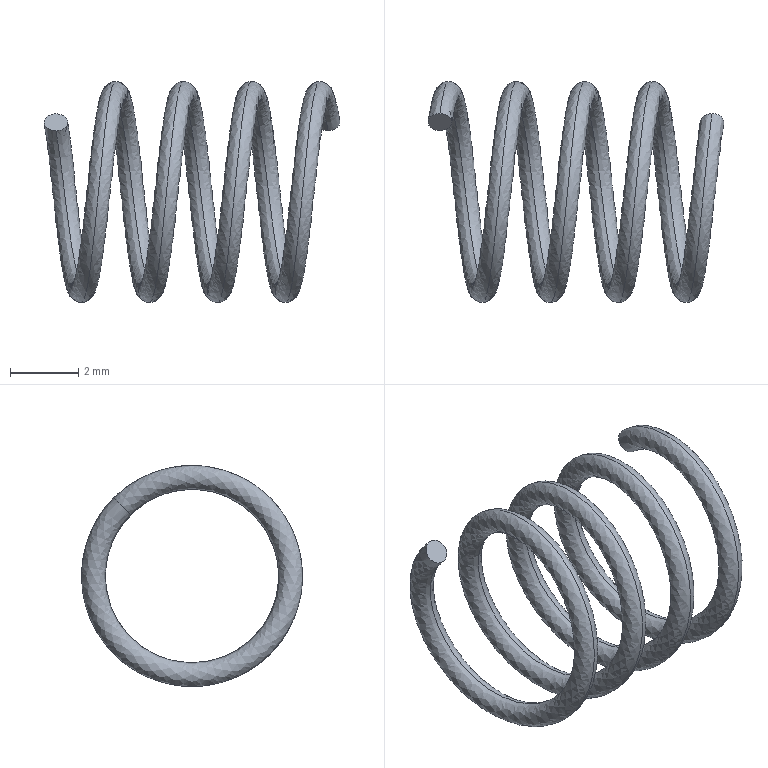Part | STEP file | High-temperature rubber spring | 1 solid | 4 faces | box 8.7 x 6.5 x 6.5 mm | volume 27.892 mm3 | spline 2 | plane 2
STEP:
#1=CARTESIAN_POINT('',(0.,0.,0.));
#2=DIRECTION('',(0.,0.,1.));
#3=DIRECTION('',(1.,0.,0.));
#4=AXIS2_PLACEMENT_3D('',#1,#2,#3);
#5=CARTESIAN_POINT('',(8.,1.803,1.803));
#6=VERTEX_POINT('',#5);
#7=CARTESIAN_POINT('',(8.,2.298,2.298));
#8=VERTEX_POINT('',#7);
#9=CARTESIAN_POINT('',(8.,1.803,1.803));
#10=CARTESIAN_POINT('',(8.7,1.803,1.803));
#11=CARTESIAN_POINT('',(8.7,2.298,2.298));
#12=CARTESIAN_POINT('',(8.,2.298,2.298));
#13=(BOUNDED_CURVE()B_SPLINE_CURVE(3,(#9,#10,#11,#12),.UNSPECIFIED.,.F.,.F.)B_SPLINE_CURVE_WITH_KNOTS((4,4),(0.,0.001094),.PIECEWISE_BEZIER_KNOTS.)CURVE()GEOMETRIC_REPRESENTATION_ITEM()RATIONAL_B_SPLINE_CURVE((1.,0.3333,0.3333,1.))REPRESENTATION_ITEM(''));
#14=CARTESIAN_POINT('',(0.,2.298,2.298));
#15=CARTESIAN_POINT('',(0.1,3.045,1.551));
#16=CARTESIAN_POINT('',(0.2,3.21,0.5084));
#17=CARTESIAN_POINT('',(0.3,3.375,-0.5346));
#18=CARTESIAN_POINT('',(0.4,2.896,-1.475));
#19=CARTESIAN_POINT('',(0.5,2.416,-2.416));
#20=CARTESIAN_POINT('',(0.6,1.475,-2.896));
#21=CARTESIAN_POINT('',(0.7,0.5346,-3.375));
#22=CARTESIAN_POINT('',(0.8,-0.5084,-3.21));
#23=CARTESIAN_POINT('',(0.9,-1.551,-3.045));
#24=CARTESIAN_POINT('',(1.,-2.298,-2.298));
#25=CARTESIAN_POINT('',(1.1,-3.045,-1.551));
#26=CARTESIAN_POINT('',(1.2,-3.21,-0.5084));
#27=CARTESIAN_POINT('',(1.3,-3.375,0.5346));
#28=CARTESIAN_POINT('',(1.4,-2.896,1.475));
#29=CARTESIAN_POINT('',(1.5,-2.416,2.416));
#30=CARTESIAN_POINT('',(1.6,-1.475,2.896));
#31=CARTESIAN_POINT('',(1.7,-0.5346,3.375));
#32=CARTESIAN_POINT('',(1.8,0.5084,3.21));
#33=CARTESIAN_POINT('',(1.9,1.551,3.045));
#34=CARTESIAN_POINT('',(2.,2.298,2.298));
#35=CARTESIAN_POINT('',(2.1,3.045,1.551));
#36=CARTESIAN_POINT('',(2.2,3.21,0.5084));
#37=CARTESIAN_POINT('',(2.3,3.375,-0.5346));
#38=CARTESIAN_POINT('',(2.4,2.896,-1.475));
#39=CARTESIAN_POINT('',(2.5,2.416,-2.416));
#40=CARTESIAN_POINT('',(2.6,1.475,-2.896));
#41=CARTESIAN_POINT('',(2.7,0.5346,-3.375));
#42=CARTESIAN_POINT('',(2.8,-0.5084,-3.21));
#43=CARTESIAN_POINT('',(2.9,-1.551,-3.045));
#44=CARTESIAN_POINT('',(3.,-2.298,-2.298));
#45=CARTESIAN_POINT('',(3.1,-3.045,-1.551));
#46=CARTESIAN_POINT('',(3.2,-3.21,-0.5084));
#47=CARTESIAN_POINT('',(3.3,-3.375,0.5346));
#48=CARTESIAN_POINT('',(3.4,-2.896,1.475));
#49=CARTESIAN_POINT('',(3.5,-2.416,2.416));
#50=CARTESIAN_POINT('',(3.6,-1.475,2.896));
#51=CARTESIAN_POINT('',(3.7,-0.5346,3.375));
#52=CARTESIAN_POINT('',(3.8,0.5084,3.21));
#53=CARTESIAN_POINT('',(3.9,1.551,3.045));
#54=CARTESIAN_POINT('',(4.,2.298,2.298));
#55=CARTESIAN_POINT('',(4.1,3.045,1.551));
#56=CARTESIAN_POINT('',(4.2,3.21,0.5084));
#57=CARTESIAN_POINT('',(4.3,3.375,-0.5346));
#58=CARTESIAN_POINT('',(4.4,2.896,-1.475));
#59=CARTESIAN_POINT('',(4.5,2.416,-2.416));
#60=CARTESIAN_POINT('',(4.6,1.475,-2.896));
#61=CARTESIAN_POINT('',(4.7,0.5346,-3.375));
#62=CARTESIAN_POINT('',(4.8,-0.5084,-3.21));
#63=CARTESIAN_POINT('',(4.9,-1.551,-3.045));
#64=CARTESIAN_POINT('',(5.,-2.298,-2.298));
#65=CARTESIAN_POINT('',(5.1,-3.045,-1.551));
#66=CARTESIAN_POINT('',(5.2,-3.21,-0.5084));
#67=CARTESIAN_POINT('',(5.3,-3.375,0.5346));
#68=CARTESIAN_POINT('',(5.4,-2.896,1.475));
#69=CARTESIAN_POINT('',(5.5,-2.416,2.416));
#70=CARTESIAN_POINT('',(5.6,-1.475,2.896));
#71=CARTESIAN_POINT('',(5.7,-0.5346,3.375));
#72=CARTESIAN_POINT('',(5.8,0.5084,3.21));
#73=CARTESIAN_POINT('',(5.9,1.551,3.045));
#74=CARTESIAN_POINT('',(6.,2.298,2.298));
#75=CARTESIAN_POINT('',(6.1,3.045,1.551));
#76=CARTESIAN_POINT('',(6.2,3.21,0.5084));
#77=CARTESIAN_POINT('',(6.3,3.375,-0.5346));
#78=CARTESIAN_POINT('',(6.4,2.896,-1.475));
#79=CARTESIAN_POINT('',(6.5,2.416,-2.416));
#80=CARTESIAN_POINT('',(6.6,1.475,-2.896));
#81=CARTESIAN_POINT('',(6.7,0.5346,-3.375));
#82=CARTESIAN_POINT('',(6.8,-0.5084,-3.21));
#83=CARTESIAN_POINT('',(6.9,-1.551,-3.045));
#84=CARTESIAN_POINT('',(7.,-2.298,-2.298));
#85=CARTESIAN_POINT('',(7.1,-3.045,-1.551));
#86=CARTESIAN_POINT('',(7.2,-3.21,-0.5084));
#87=CARTESIAN_POINT('',(7.3,-3.375,0.5346));
#88=CARTESIAN_POINT('',(7.4,-2.896,1.475));
#89=CARTESIAN_POINT('',(7.5,-2.416,2.416));
#90=CARTESIAN_POINT('',(7.6,-1.475,2.896));
#91=CARTESIAN_POINT('',(7.7,-0.5346,3.375));
#92=CARTESIAN_POINT('',(7.8,0.5084,3.21));
#93=CARTESIAN_POINT('',(7.9,1.551,3.045));
#94=CARTESIAN_POINT('',(8.,2.298,2.298));
#95=CARTESIAN_POINT('',(0.7,2.298,2.298));
#96=CARTESIAN_POINT('',(0.8,3.045,1.551));
#97=CARTESIAN_POINT('',(0.9,3.21,0.5084));
#98=CARTESIAN_POINT('',(1.,3.375,-0.5346));
#99=CARTESIAN_POINT('',(1.1,2.896,-1.475));
#100=CARTESIAN_POINT('',(1.2,2.416,-2.416));
#101=CARTESIAN_POINT('',(1.3,1.475,-2.896));
#102=CARTESIAN_POINT('',(1.4,0.5346,-3.375));
#103=CARTESIAN_POINT('',(1.5,-0.5084,-3.21));
#104=CARTESIAN_POINT('',(1.6,-1.551,-3.045));
#105=CARTESIAN_POINT('',(1.7,-2.298,-2.298));
#106=CARTESIAN_POINT('',(1.8,-3.045,-1.551));
#107=CARTESIAN_POINT('',(1.9,-3.21,-0.5084));
#108=CARTESIAN_POINT('',(2.,-3.375,0.5346));
#109=CARTESIAN_POINT('',(2.1,-2.896,1.475));
#110=CARTESIAN_POINT('',(2.2,-2.416,2.416));
#111=CARTESIAN_POINT('',(2.3,-1.475,2.896));
#112=CARTESIAN_POINT('',(2.4,-0.5346,3.375));
#113=CARTESIAN_POINT('',(2.5,0.5084,3.21));
#114=CARTESIAN_POINT('',(2.6,1.551,3.045));
#115=CARTESIAN_POINT('',(2.7,2.298,2.298));
#116=CARTESIAN_POINT('',(2.8,3.045,1.551));
#117=CARTESIAN_POINT('',(2.9,3.21,0.5084));
#118=CARTESIAN_POINT('',(3.,3.375,-0.5346));
#119=CARTESIAN_POINT('',(3.1,2.896,-1.475));
#120=CARTESIAN_POINT('',(3.2,2.416,-2.416));
#121=CARTESIAN_POINT('',(3.3,1.475,-2.896));
#122=CARTESIAN_POINT('',(3.4,0.5346,-3.375));
#123=CARTESIAN_POINT('',(3.5,-0.5084,-3.21));
#124=CARTESIAN_POINT('',(3.6,-1.551,-3.045));
#125=CARTESIAN_POINT('',(3.7,-2.298,-2.298));
#126=CARTESIAN_POINT('',(3.8,-3.045,-1.551));
#127=CARTESIAN_POINT('',(3.9,-3.21,-0.5084));
#128=CARTESIAN_POINT('',(4.,-3.375,0.5346));
#129=CARTESIAN_POINT('',(4.1,-2.896,1.475));
#130=CARTESIAN_POINT('',(4.2,-2.416,2.416));
#131=CARTESIAN_POINT('',(4.3,-1.475,2.896));
#132=CARTESIAN_POINT('',(4.4,-0.5346,3.375));
#133=CARTESIAN_POINT('',(4.5,0.5084,3.21));
#134=CARTESIAN_POINT('',(4.6,1.551,3.045));
#135=CARTESIAN_POINT('',(4.7,2.298,2.298));
#136=CARTESIAN_POINT('',(4.8,3.045,1.551));
#137=CARTESIAN_POINT('',(4.9,3.21,0.5084));
#138=CARTESIAN_POINT('',(5.,3.375,-0.5346));
#139=CARTESIAN_POINT('',(5.1,2.896,-1.475));
#140=CARTESIAN_POINT('',(5.2,2.416,-2.416));
#141=CARTESIAN_POINT('',(5.3,1.475,-2.896));
#142=CARTESIAN_POINT('',(5.4,0.5346,-3.375));
#143=CARTESIAN_POINT('',(5.5,-0.5084,-3.21));
#144=CARTESIAN_POINT('',(5.6,-1.551,-3.045));
#145=CARTESIAN_POINT('',(5.7,-2.298,-2.298));
#146=CARTESIAN_POINT('',(5.8,-3.045,-1.551));
#147=CARTESIAN_POINT('',(5.9,-3.21,-0.5084));
#148=CARTESIAN_POINT('',(6.,-3.375,0.5346));
#149=CARTESIAN_POINT('',(6.1,-2.896,1.475));
#150=CARTESIAN_POINT('',(6.2,-2.416,2.416));
#151=CARTESIAN_POINT('',(6.3,-1.475,2.896));
#152=CARTESIAN_POINT('',(6.4,-0.5346,3.375));
#153=CARTESIAN_POINT('',(6.5,0.5084,3.21));
#154=CARTESIAN_POINT('',(6.6,1.551,3.045));
#155=CARTESIAN_POINT('',(6.7,2.298,2.298));
#156=CARTESIAN_POINT('',(6.8,3.045,1.551));
#157=CARTESIAN_POINT('',(6.9,3.21,0.5084));
#158=CARTESIAN_POINT('',(7.,3.375,-0.5346));
#159=CARTESIAN_POINT('',(7.1,2.896,-1.475));
#160=CARTESIAN_POINT('',(7.2,2.416,-2.416));
#161=CARTESIAN_POINT('',(7.3,1.475,-2.896));
#162=CARTESIAN_POINT('',(7.4,0.5346,-3.375));
#163=CARTESIAN_POINT('',(7.5,-0.5084,-3.21));
#164=CARTESIAN_POINT('',(7.6,-1.551,-3.045));
#165=CARTESIAN_POINT('',(7.7,-2.298,-2.298));
#166=CARTESIAN_POINT('',(7.8,-3.045,-1.551));
#167=CARTESIAN_POINT('',(7.9,-3.21,-0.5084));
#168=CARTESIAN_POINT('',(8.,-3.375,0.5346));
#169=CARTESIAN_POINT('',(8.1,-2.896,1.475));
#170=CARTESIAN_POINT('',(8.2,-2.416,2.416));
#171=CARTESIAN_POINT('',(8.3,-1.475,2.896));
#172=CARTESIAN_POINT('',(8.4,-0.5346,3.375));
#173=CARTESIAN_POINT('',(8.5,0.5084,3.21));
#174=CARTESIAN_POINT('',(8.6,1.551,3.045));
#175=CARTESIAN_POINT('',(8.7,2.298,2.298));
#176=CARTESIAN_POINT('',(0.7,1.803,1.803));
#177=CARTESIAN_POINT('',(0.8,2.389,1.217));
#178=CARTESIAN_POINT('',(0.9,2.519,0.3989));
#179=CARTESIAN_POINT('',(1.,2.648,-0.4194));
#180=CARTESIAN_POINT('',(1.1,2.272,-1.158));
#181=CARTESIAN_POINT('',(1.2,1.896,-1.896));
#182=CARTESIAN_POINT('',(1.3,1.158,-2.272));
#183=CARTESIAN_POINT('',(1.4,0.4194,-2.648));
#184=CARTESIAN_POINT('',(1.5,-0.3989,-2.519));
#185=CARTESIAN_POINT('',(1.6,-1.217,-2.389));
#186=CARTESIAN_POINT('',(1.7,-1.803,-1.803));
#187=CARTESIAN_POINT('',(1.8,-2.389,-1.217));
#188=CARTESIAN_POINT('',(1.9,-2.519,-0.3989));
#189=CARTESIAN_POINT('',(2.,-2.648,0.4194));
#190=CARTESIAN_POINT('',(2.1,-2.272,1.158));
#191=CARTESIAN_POINT('',(2.2,-1.896,1.896));
#192=CARTESIAN_POINT('',(2.3,-1.158,2.272));
#193=CARTESIAN_POINT('',(2.4,-0.4194,2.648));
#194=CARTESIAN_POINT('',(2.5,0.3989,2.519));
#195=CARTESIAN_POINT('',(2.6,1.217,2.389));
#196=CARTESIAN_POINT('',(2.7,1.803,1.803));
#197=CARTESIAN_POINT('',(2.8,2.389,1.217));
#198=CARTESIAN_POINT('',(2.9,2.519,0.3989));
#199=CARTESIAN_POINT('',(3.,2.648,-0.4194));
#200=CARTESIAN_POINT('',(3.1,2.272,-1.158));
#201=CARTESIAN_POINT('',(3.2,1.896,-1.896));
#202=CARTESIAN_POINT('',(3.3,1.158,-2.272));
#203=CARTESIAN_POINT('',(3.4,0.4194,-2.648));
#204=CARTESIAN_POINT('',(3.5,-0.3989,-2.519));
#205=CARTESIAN_POINT('',(3.6,-1.217,-2.389));
#206=CARTESIAN_POINT('',(3.7,-1.803,-1.803));
#207=CARTESIAN_POINT('',(3.8,-2.389,-1.217));
#208=CARTESIAN_POINT('',(3.9,-2.519,-0.3989));
#209=CARTESIAN_POINT('',(4.,-2.648,0.4194));
#210=CARTESIAN_POINT('',(4.1,-2.272,1.158));
#211=CARTESIAN_POINT('',(4.2,-1.896,1.896));
#212=CARTESIAN_POINT('',(4.3,-1.158,2.272));
#213=CARTESIAN_POINT('',(4.4,-0.4194,2.648));
#214=CARTESIAN_POINT('',(4.5,0.3989,2.519));
#215=CARTESIAN_POINT('',(4.6,1.217,2.389));
#216=CARTESIAN_POINT('',(4.7,1.803,1.803));
#217=CARTESIAN_POINT('',(4.8,2.389,1.217));
#218=CARTESIAN_POINT('',(4.9,2.519,0.3989));
#219=CARTESIAN_POINT('',(5.,2.648,-0.4194));
#220=CARTESIAN_POINT('',(5.1,2.272,-1.158));
#221=CARTESIAN_POINT('',(5.2,1.896,-1.896));
#222=CARTESIAN_POINT('',(5.3,1.158,-2.272));
#223=CARTESIAN_POINT('',(5.4,0.4194,-2.648));
#224=CARTESIAN_POINT('',(5.5,-0.3989,-2.519));
#225=CARTESIAN_POINT('',(5.6,-1.217,-2.389));
#226=CARTESIAN_POINT('',(5.7,-1.803,-1.803));
#227=CARTESIAN_POINT('',(5.8,-2.389,-1.217));
#228=CARTESIAN_POINT('',(5.9,-2.519,-0.3989));
#229=CARTESIAN_POINT('',(6.,-2.648,0.4194));
#230=CARTESIAN_POINT('',(6.1,-2.272,1.158));
#231=CARTESIAN_POINT('',(6.2,-1.896,1.896));
#232=CARTESIAN_POINT('',(6.3,-1.158,2.272));
#233=CARTESIAN_POINT('',(6.4,-0.4194,2.648));
#234=CARTESIAN_POINT('',(6.5,0.3989,2.519));
#235=CARTESIAN_POINT('',(6.6,1.217,2.389));
#236=CARTESIAN_POINT('',(6.7,1.803,1.803));
#237=CARTESIAN_POINT('',(6.8,2.389,1.217));
#238=CARTESIAN_POINT('',(6.9,2.519,0.3989));
#239=CARTESIAN_POINT('',(7.,2.648,-0.4194));
#240=CARTESIAN_POINT('',(7.1,2.272,-1.158));
#241=CARTESIAN_POINT('',(7.2,1.896,-1.896));
#242=CARTESIAN_POINT('',(7.3,1.158,-2.272));
#243=CARTESIAN_POINT('',(7.4,0.4194,-2.648));
#244=CARTESIAN_POINT('',(7.5,-0.3989,-2.519));
#245=CARTESIAN_POINT('',(7.6,-1.217,-2.389));
#246=CARTESIAN_POINT('',(7.7,-1.803,-1.803));
#247=CARTESIAN_POINT('',(7.8,-2.389,-1.217));
#248=CARTESIAN_POINT('',(7.9,-2.519,-0.3989));
#249=CARTESIAN_POINT('',(8.,-2.648,0.4194));
#250=CARTESIAN_POINT('',(8.1,-2.272,1.158));
#251=CARTESIAN_POINT('',(8.2,-1.896,1.896));
#252=CARTESIAN_POINT('',(8.3,-1.158,2.272));
#253=CARTESIAN_POINT('',(8.4,-0.4194,2.648));
#254=CARTESIAN_POINT('',(8.5,0.3989,2.519));
#255=CARTESIAN_POINT('',(8.6,1.217,2.389));
#256=CARTESIAN_POINT('',(8.7,1.803,1.803));
#257=CARTESIAN_POINT('',(0.,1.803,1.803));
#258=CARTESIAN_POINT('',(0.1,2.389,1.217));
#259=CARTESIAN_POINT('',(0.2,2.519,0.3989));
#260=CARTESIAN_POINT('',(0.3,2.648,-0.4194));
#261=CARTESIAN_POINT('',(0.4,2.272,-1.158));
#262=CARTESIAN_POINT('',(0.5,1.896,-1.896));
#263=CARTESIAN_POINT('',(0.6,1.158,-2.272));
#264=CARTESIAN_POINT('',(0.7,0.4194,-2.648));
#265=CARTESIAN_POINT('',(0.8,-0.3989,-2.519));
#266=CARTESIAN_POINT('',(0.9,-1.217,-2.389));
#267=CARTESIAN_POINT('',(1.,-1.803,-1.803));
#268=CARTESIAN_POINT('',(1.1,-2.389,-1.217));
#269=CARTESIAN_POINT('',(1.2,-2.519,-0.3989));
#270=CARTESIAN_POINT('',(1.3,-2.648,0.4194));
#271=CARTESIAN_POINT('',(1.4,-2.272,1.158));
#272=CARTESIAN_POINT('',(1.5,-1.896,1.896));
#273=CARTESIAN_POINT('',(1.6,-1.158,2.272));
#274=CARTESIAN_POINT('',(1.7,-0.4194,2.648));
#275=CARTESIAN_POINT('',(1.8,0.3989,2.519));
#276=CARTESIAN_POINT('',(1.9,1.217,2.389));
#277=CARTESIAN_POINT('',(2.,1.803,1.803));
#278=CARTESIAN_POINT('',(2.1,2.389,1.217));
#279=CARTESIAN_POINT('',(2.2,2.519,0.3989));
#280=CARTESIAN_POINT('',(2.3,2.648,-0.4194));
#281=CARTESIAN_POINT('',(2.4,2.272,-1.158));
#282=CARTESIAN_POINT('',(2.5,1.896,-1.896));
#283=CARTESIAN_POINT('',(2.6,1.158,-2.272));
#284=CARTESIAN_POINT('',(2.7,0.4194,-2.648));
#285=CARTESIAN_POINT('',(2.8,-0.3989,-2.519));
#286=CARTESIAN_POINT('',(2.9,-1.217,-2.389));
#287=CARTESIAN_POINT('',(3.,-1.803,-1.803));
#288=CARTESIAN_POINT('',(3.1,-2.389,-1.217));
#289=CARTESIAN_POINT('',(3.2,-2.519,-0.3989));
#290=CARTESIAN_POINT('',(3.3,-2.648,0.4194));
#291=CARTESIAN_POINT('',(3.4,-2.272,1.158));
#292=CARTESIAN_POINT('',(3.5,-1.896,1.896));
#293=CARTESIAN_POINT('',(3.6,-1.158,2.272));
#294=CARTESIAN_POINT('',(3.7,-0.4194,2.648));
#295=CARTESIAN_POINT('',(3.8,0.3989,2.519));
#296=CARTESIAN_POINT('',(3.9,1.217,2.389));
#297=CARTESIAN_POINT('',(4.,1.803,1.803));
#298=CARTESIAN_POINT('',(4.1,2.389,1.217));
#299=CARTESIAN_POINT('',(4.2,2.519,0.3989));
#300=CARTESIAN_POINT('',(4.3,2.648,-0.4194));
#301=CARTESIAN_POINT('',(4.4,2.272,-1.158));
#302=CARTESIAN_POINT('',(4.5,1.896,-1.896));
#303=CARTESIAN_POINT('',(4.6,1.158,-2.272));
#304=CARTESIAN_POINT('',(4.7,0.4194,-2.648));
#305=CARTESIAN_POINT('',(4.8,-0.3989,-2.519));
#306=CARTESIAN_POINT('',(4.9,-1.217,-2.389));
#307=CARTESIAN_POINT('',(5.,-1.803,-1.803));
#308=CARTESIAN_POINT('',(5.1,-2.389,-1.217));
#309=CARTESIAN_POINT('',(5.2,-2.519,-0.3989));
#310=CARTESIAN_POINT('',(5.3,-2.648,0.4194));
#311=CARTESIAN_POINT('',(5.4,-2.272,1.158));
#312=CARTESIAN_POINT('',(5.5,-1.896,1.896));
#313=CARTESIAN_POINT('',(5.6,-1.158,2.272));
#314=CARTESIAN_POINT('',(5.7,-0.4194,2.648));
#315=CARTESIAN_POINT('',(5.8,0.3989,2.519));
#316=CARTESIAN_POINT('',(5.9,1.217,2.389));
#317=CARTESIAN_POINT('',(6.,1.803,1.803));
#318=CARTESIAN_POINT('',(6.1,2.389,1.217));
#319=CARTESIAN_POINT('',(6.2,2.519,0.3989));
#320=CARTESIAN_POINT('',(6.3,2.648,-0.4194));
#321=CARTESIAN_POINT('',(6.4,2.272,-1.158));
#322=CARTESIAN_POINT('',(6.5,1.896,-1.896));
#323=CARTESIAN_POINT('',(6.6,1.158,-2.272));
#324=CARTESIAN_POINT('',(6.7,0.4194,-2.648));
#325=CARTESIAN_POINT('',(6.8,-0.3989,-2.519));
#326=CARTESIAN_POINT('',(6.9,-1.217,-2.389));
#327=CARTESIAN_POINT('',(7.,-1.803,-1.803));
#328=CARTESIAN_POINT('',(7.1,-2.389,-1.217));
#329=CARTESIAN_POINT('',(7.2,-2.519,-0.3989));
#330=CARTESIAN_POINT('',(7.3,-2.648,0.4194));
#331=CARTESIAN_POINT('',(7.4,-2.272,1.158));
#332=CARTESIAN_POINT('',(7.5,-1.896,1.896));
#333=CARTESIAN_POINT('',(7.6,-1.158,2.272));
#334=CARTESIAN_POINT('',(7.7,-0.4194,2.648));
#335=CARTESIAN_POINT('',(7.8,0.3989,2.519));
#336=CARTESIAN_POINT('',(7.9,1.217,2.389));
#337=CARTESIAN_POINT('',(8.,1.803,1.803));
#338=(BOUNDED_SURFACE()B_SPLINE_SURFACE(3,2,((#14,#15,#16,#17,#18,#19,#20,#21,#22,#23,#24,#25,#26,#27,#28,#29,#30,#31,#32,#33,#34,#35,#36,#37,#38,#39,#40,#41,#42,#43,#44,#45,#46,#47,#48,#49,#50,#51,#52,#53,#54,#55,#56,#57,#58,#59,#60,#61,#62,#63,#64,#65,#66,#67,#68,#69,#70,#71,#72,#73,#74,#75,#76,#77,#78,#79,#80,#81,#82,#83,#84,#85,#86,#87,#88,#89,#90,#91,#92,#93,#94),(#95,#96,#97,#98,#99,#100,#101,#102,#103,#104,#105,#106,#107,#108,#109,#110,#111,#112,#113,#114,#115,#116,#117,#118,#119,#120,#121,#122,#123,#124,#125,#126,#127,#128,#129,#130,#131,#132,#133,#134,#135,#136,#137,#138,#139,#140,#141,#142,#143,#144,#145,#146,#147,#148,#149,#150,#151,#152,#153,#154,#155,#156,#157,#158,#159,#160,#161,#162,#163,#164,#165,#166,#167,#168,#169,#170,#171,#172,#173,#174,#175),(#176,#177,#178,#179,#180,#181,#182,#183,#184,#185,#186,#187,#188,#189,#190,#191,#192,#193,#194,#195,#196,#197,#198,#199,#200,#201,#202,#203,#204,#205,#206,#207,#208,#209,#210,#211,#212,#213,#214,#215,#216,#217,#218,#219,#220,#221,#222,#223,#224,#225,#226,#227,#228,#229,#230,#231,#232,#233,#234,#235,#236,#237,#238,#239,#240,#241,#242,#243,#244,#245,#246,#247,#248,#249,#250,#251,#252,#253,#254,#255,#256),(#257,#258,#259,#260,#261,#262,#263,#264,#265,#266,#267,#268,#269,#270,#271,#272,#273,#274,#275,#276,#277,#278,#279,#280,#281,#282,#283,#284,#285,#286,#287,#288,#289,#290,#291,#292,#293,#294,#295,#296,#297,#298,#299,#300,#301,#302,#303,#304,#305,#306,#307,#308,#309,#310,#311,#312,#313,#314,#315,#316,#317,#318,#319,#320,#321,#322,#323,#324,#325,#326,#327,#328,#329,#330,#331,#332,#333,#334,#335,#336,#337)),.UNSPECIFIED.,.F.,.F.,.F.)B_SPLINE_SURFACE_WITH_KNOTS((4,4),(3,2,2,2,2,2,2,2,2,2,2,2,2,2,2,2,2,2,2,2,2,2,2,2,2,2,2,2,2,2,2,2,2,2,2,2,2,2,2,2,3),(0.,0.5),(0.,0.025,0.05,0.075,0.1,0.125,0.15,0.175,0.2,0.225,0.25,0.275,0.3,0.325,0.35,0.375,0.4,0.425,0.45,0.475,0.5,0.525,0.55,0.575,0.6,0.625,0.65,0.675,0.7,0.725,0.75,0.775,0.8,0.825,0.85,0.875,0.9,0.925,0.95,0.975,1.),.PIECEWISE_BEZIER_KNOTS.)GEOMETRIC_REPRESENTATION_ITEM()RATIONAL_B_SPLINE_SURFACE(((1.,0.9511,1.,0.9511,1.,0.9511,1.,0.9511,1.,0.9511,1.,0.9511,1.,0.9511,1.,0.9511,1.,0.9511,1.,0.9511,1.,0.9511,1.,0.9511,1.,0.9511,1.,0.9511,1.,0.9511,1.,0.9511,1.,0.9511,1.,0.9511,1.,0.9511,1.,0.9511,1.,0.9511,1.,0.9511,1.,0.9511,1.,0.9511,1.,0.9511,1.,0.9511,1.,0.9511,1.,0.9511,1.,0.9511,1.,0.9511,1.,0.9511,1.,0.9511,1.,0.9511,1.,0.9511,1.,0.9511,1.,0.9511,1.,0.9511,1.,0.9511,1.,0.9511,1.,0.9511,1.),(0.3333,0.317,0.3333,0.317,0.3333,0.317,0.3333,0.317,0.3333,0.317,0.3333,0.317,0.3333,0.317,0.3333,0.317,0.3333,0.317,0.3333,0.317,0.3333,0.317,0.3333,0.317,0.3333,0.317,0.3333,0.317,0.3333,0.317,0.3333,0.317,0.3333,0.317,0.3333,0.317,0.3333,0.317,0.3333,0.317,0.3333,0.317,0.3333,0.317,0.3333,0.317,0.3333,0.317,0.3333,0.317,0.3333,0.317,0.3333,0.317,0.3333,0.317,0.3333,0.317,0.3333,0.317,0.3333,0.317,0.3333,0.317,0.3333,0.317,0.3333,0.317,0.3333,0.317,0.3333,0.317,0.3333,0.317,0.3333,0.317,0.3333,0.317,0.3333,0.317,0.3333),(0.3333,0.317,0.3333,0.317,0.3333,0.317,0.3333,0.317,0.3333,0.317,0.3333,0.317,0.3333,0.317,0.3333,0.317,0.3333,0.317,0.3333,0.317,0.3333,0.317,0.3333,0.317,0.3333,0.317,0.3333,0.317,0.3333,0.317,0.3333,0.317,0.3333,0.317,0.3333,0.317,0.3333,0.317,0.3333,0.317,0.3333,0.317,0.3333,0.317,0.3333,0.317,0.3333,0.317,0.3333,0.317,0.3333,0.317,0.3333,0.317,0.3333,0.317,0.3333,0.317,0.3333,0.317,0.3333,0.317,0.3333,0.317,0.3333,0.317,0.3333,0.317,0.3333,0.317,0.3333,0.317,0.3333,0.317,0.3333,0.317,0.3333,0.317,0.3333,0.317,0.3333),(1.,0.9511,1.,0.9511,1.,0.9511,1.,0.9511,1.,0.9511,1.,0.9511,1.,0.9511,1.,0.9511,1.,0.9511,1.,0.9511,1.,0.9511,1.,0.9511,1.,0.9511,1.,0.9511,1.,0.9511,1.,0.9511,1.,0.9511,1.,0.9511,1.,0.9511,1.,0.9511,1.,0.9511,1.,0.9511,1.,0.9511,1.,0.9511,1.,0.9511,1.,0.9511,1.,0.9511,1.,0.9511,1.,0.9511,1.,0.9511,1.,0.9511,1.,0.9511,1.,0.9511,1.,0.9511,1.,0.9511,1.,0.9511,1.,0.9511,1.,0.9511,1.,0.9511,1.,0.9511,1.)))REPRESENTATION_ITEM('')SURFACE());
#339=CARTESIAN_POINT('',(0.5,1.));
#340=CARTESIAN_POINT('',(0.,1.));
#341=B_SPLINE_CURVE_WITH_KNOTS('',1,(#339,#340),.UNSPECIFIED.,.F.,.F.,(2,2),(0.,0.001094),.PIECEWISE_BEZIER_KNOTS.);
#342=(GEOMETRIC_REPRESENTATION_CONTEXT(2)PARAMETRIC_REPRESENTATION_CONTEXT()REPRESENTATION_CONTEXT('',''));
#343=DEFINITIONAL_REPRESENTATION('',(#341),#342);
#344=PCURVE('',#338,#343);
#345=CARTESIAN_POINT('',(7.646,2.301,2.301));
#346=DIRECTION('',(0.,-0.7071,0.7071));
#347=DIRECTION('',(0.,-0.7071,-0.7071));
#348=AXIS2_PLACEMENT_3D('',#345,#346,#347);
#349=PLANE('',#348);
#350=CARTESIAN_POINT('',(0.7042,0.3542));
#351=CARTESIAN_POINT('',(0.7042,1.054));
#352=CARTESIAN_POINT('',(0.0042,1.054));
#353=CARTESIAN_POINT('',(0.0042,0.3542));
#354=(BOUNDED_CURVE()B_SPLINE_CURVE(3,(#350,#351,#352,#353),.UNSPECIFIED.,.F.,.F.)B_SPLINE_CURVE_WITH_KNOTS((4,4),(0.,0.001094),.PIECEWISE_BEZIER_KNOTS.)CURVE()GEOMETRIC_REPRESENTATION_ITEM()RATIONAL_B_SPLINE_CURVE((1.,0.3333,0.3333,1.))REPRESENTATION_ITEM(''));
#355=(GEOMETRIC_REPRESENTATION_CONTEXT(2)PARAMETRIC_REPRESENTATION_CONTEXT()REPRESENTATION_CONTEXT('',''));
#356=DEFINITIONAL_REPRESENTATION('',(#354),#355);
#357=PCURVE('',#349,#356);
#358=SURFACE_CURVE('',#13,(#344,#357),.PCURVE_S1.);
#359=EDGE_CURVE('',#6,#8,#358,.T.);
#360=ORIENTED_EDGE('',*,*,#359,.T.);
#361=CARTESIAN_POINT('',(0.,2.298,2.298));
#362=VERTEX_POINT('',#361);
#363=CARTESIAN_POINT('',(8.,2.298,2.298));
#364=CARTESIAN_POINT('',(7.9,1.551,3.045));
#365=CARTESIAN_POINT('',(7.8,0.5084,3.21));
#366=CARTESIAN_POINT('',(7.7,-0.5346,3.375));
#367=CARTESIAN_POINT('',(7.6,-1.475,2.896));
#368=CARTESIAN_POINT('',(7.5,-2.416,2.416));
#369=CARTESIAN_POINT('',(7.4,-2.896,1.475));
#370=CARTESIAN_POINT('',(7.3,-3.375,0.5346));
#371=CARTESIAN_POINT('',(7.2,-3.21,-0.5084));
#372=CARTESIAN_POINT('',(7.1,-3.045,-1.551));
#373=CARTESIAN_POINT('',(7.,-2.298,-2.298));
#374=CARTESIAN_POINT('',(6.9,-1.551,-3.045));
#375=CARTESIAN_POINT('',(6.8,-0.5084,-3.21));
#376=CARTESIAN_POINT('',(6.7,0.5346,-3.375));
#377=CARTESIAN_POINT('',(6.6,1.475,-2.896));
#378=CARTESIAN_POINT('',(6.5,2.416,-2.416));
#379=CARTESIAN_POINT('',(6.4,2.896,-1.475));
#380=CARTESIAN_POINT('',(6.3,3.375,-0.5346));
#381=CARTESIAN_POINT('',(6.2,3.21,0.5084));
#382=CARTESIAN_POINT('',(6.1,3.045,1.551));
#383=CARTESIAN_POINT('',(6.,2.298,2.298));
#384=CARTESIAN_POINT('',(5.9,1.551,3.045));
#385=CARTESIAN_POINT('',(5.8,0.5084,3.21));
#386=CARTESIAN_POINT('',(5.7,-0.5346,3.375));
#387=CARTESIAN_POINT('',(5.6,-1.475,2.896));
#388=CARTESIAN_POINT('',(5.5,-2.416,2.416));
#389=CARTESIAN_POINT('',(5.4,-2.896,1.475));
#390=CARTESIAN_POINT('',(5.3,-3.375,0.5346));
#391=CARTESIAN_POINT('',(5.2,-3.21,-0.5084));
#392=CARTESIAN_POINT('',(5.1,-3.045,-1.551));
#393=CARTESIAN_POINT('',(5.,-2.298,-2.298));
#394=CARTESIAN_POINT('',(4.9,-1.551,-3.045));
#395=CARTESIAN_POINT('',(4.8,-0.5084,-3.21));
#396=CARTESIAN_POINT('',(4.7,0.5346,-3.375));
#397=CARTESIAN_POINT('',(4.6,1.475,-2.896));
#398=CARTESIAN_POINT('',(4.5,2.416,-2.416));
#399=CARTESIAN_POINT('',(4.4,2.896,-1.475));
#400=CARTESIAN_POINT('',(4.3,3.375,-0.5346));
#401=CARTESIAN_POINT('',(4.2,3.21,0.5084));
#402=CARTESIAN_POINT('',(4.1,3.045,1.551));
#403=CARTESIAN_POINT('',(4.,2.298,2.298));
#404=CARTESIAN_POINT('',(3.9,1.551,3.045));
#405=CARTESIAN_POINT('',(3.8,0.5084,3.21));
#406=CARTESIAN_POINT('',(3.7,-0.5346,3.375));
#407=CARTESIAN_POINT('',(3.6,-1.475,2.896));
#408=CARTESIAN_POINT('',(3.5,-2.416,2.416));
#409=CARTESIAN_POINT('',(3.4,-2.896,1.475));
#410=CARTESIAN_POINT('',(3.3,-3.375,0.5346));
#411=CARTESIAN_POINT('',(3.2,-3.21,-0.5084));
#412=CARTESIAN_POINT('',(3.1,-3.045,-1.551));
#413=CARTESIAN_POINT('',(3.,-2.298,-2.298));
#414=CARTESIAN_POINT('',(2.9,-1.551,-3.045));
#415=CARTESIAN_POINT('',(2.8,-0.5084,-3.21));
#416=CARTESIAN_POINT('',(2.7,0.5346,-3.375));
#417=CARTESIAN_POINT('',(2.6,1.475,-2.896));
#418=CARTESIAN_POINT('',(2.5,2.416,-2.416));
#419=CARTESIAN_POINT('',(2.4,2.896,-1.475));
#420=CARTESIAN_POINT('',(2.3,3.375,-0.5346));
#421=CARTESIAN_POINT('',(2.2,3.21,0.5084));
#422=CARTESIAN_POINT('',(2.1,3.045,1.551));
#423=CARTESIAN_POINT('',(2.,2.298,2.298));
#424=CARTESIAN_POINT('',(1.9,1.551,3.045));
#425=CARTESIAN_POINT('',(1.8,0.5084,3.21));
#426=CARTESIAN_POINT('',(1.7,-0.5346,3.375));
#427=CARTESIAN_POINT('',(1.6,-1.475,2.896));
#428=CARTESIAN_POINT('',(1.5,-2.416,2.416));
#429=CARTESIAN_POINT('',(1.4,-2.896,1.475));
#430=CARTESIAN_POINT('',(1.3,-3.375,0.5346));
#431=CARTESIAN_POINT('',(1.2,-3.21,-0.5084));
#432=CARTESIAN_POINT('',(1.1,-3.045,-1.551));
#433=CARTESIAN_POINT('',(1.,-2.298,-2.298));
#434=CARTESIAN_POINT('',(0.9,-1.551,-3.045));
#435=CARTESIAN_POINT('',(0.8,-0.5084,-3.21));
#436=CARTESIAN_POINT('',(0.7,0.5346,-3.375));
#437=CARTESIAN_POINT('',(0.6,1.475,-2.896));
#438=CARTESIAN_POINT('',(0.5,2.416,-2.416));
#439=CARTESIAN_POINT('',(0.4,2.896,-1.475));
#440=CARTESIAN_POINT('',(0.3,3.375,-0.5346));
#441=CARTESIAN_POINT('',(0.2,3.21,0.5084));
#442=CARTESIAN_POINT('',(0.1,3.045,1.551));
#443=CARTESIAN_POINT('',(0.,2.298,2.298));
#444=(BOUNDED_CURVE()B_SPLINE_CURVE(2,(#363,#364,#365,#366,#367,#368,#369,#370,#371,#372,#373,#374,#375,#376,#377,#378,#379,#380,#381,#382,#383,#384,#385,#386,#387,#388,#389,#390,#391,#392,#393,#394,#395,#396,#397,#398,#399,#400,#401,#402,#403,#404,#405,#406,#407,#408,#409,#410,#411,#412,#413,#414,#415,#416,#417,#418,#419,#420,#421,#422,#423,#424,#425,#426,#427,#428,#429,#430,#431,#432,#433,#434,#435,#436,#437,#438,#439,#440,#441,#442,#443),.UNSPECIFIED.,.F.,.F.)B_SPLINE_CURVE_WITH_KNOTS((3,2,2,2,2,2,2,2,2,2,2,2,2,2,2,2,2,2,2,2,2,2,2,2,2,2,2,2,2,2,2,2,2,2,2,2,2,2,2,2,3),(0.,0.025,0.05,0.075,0.1,0.125,0.15,0.175,0.2,0.225,0.25,0.275,0.3,0.325,0.35,0.375,0.4,0.425,0.45,0.475,0.5,0.525,0.55,0.575,0.6,0.625,0.65,0.675,0.7,0.725,0.75,0.775,0.8,0.825,0.85,0.875,0.9,0.925,0.95,0.975,1.),.UNSPECIFIED.)CURVE()GEOMETRIC_REPRESENTATION_ITEM()RATIONAL_B_SPLINE_CURVE((1.,0.9511,1.,0.9511,1.,0.9511,1.,0.9511,1.,0.9511,1.,0.9511,1.,0.9511,1.,0.9511,1.,0.9511,1.,0.9511,1.,0.9511,1.,0.9511,1.,0.9511,1.,0.9511,1.,0.9511,1.,0.9511,1.,0.9511,1.,0.9511,1.,0.9511,1.,0.9511,1.,0.9511,1.,0.9511,1.,0.9511,1.,0.9511,1.,0.9511,1.,0.9511,1.,0.9511,1.,0.9511,1.,0.9511,1.,0.9511,1.,0.9511,1.,0.9511,1.,0.9511,1.,0.9511,1.,0.9511,1.,0.9511,1.,0.9511,1.,0.9511,1.,0.9511,1.,0.9511,1.))REPRESENTATION_ITEM(''));
#445=CARTESIAN_POINT('',(0.,1.));
#446=DIRECTION('',(0.,-1.));
#447=VECTOR('',#446,1.);
#448=LINE('',#445,#447);
#449=(GEOMETRIC_REPRESENTATION_CONTEXT(2)PARAMETRIC_REPRESENTATION_CONTEXT()REPRESENTATION_CONTEXT('',''));
#450=DEFINITIONAL_REPRESENTATION('',(#448),#449);
#451=PCURVE('',#338,#450);
#452=CARTESIAN_POINT('',(0.,1.803,1.803));
#453=CARTESIAN_POINT('',(0.1,2.389,1.217));
#454=CARTESIAN_POINT('',(0.2,2.519,0.3989));
#455=CARTESIAN_POINT('',(0.3,2.648,-0.4194));
#456=CARTESIAN_POINT('',(0.4,2.272,-1.158));
#457=CARTESIAN_POINT('',(0.5,1.896,-1.896));
#458=CARTESIAN_POINT('',(0.6,1.158,-2.272));
#459=CARTESIAN_POINT('',(0.7,0.4194,-2.648));
#460=CARTESIAN_POINT('',(0.8,-0.3989,-2.519));
#461=CARTESIAN_POINT('',(0.9,-1.217,-2.389));
#462=CARTESIAN_POINT('',(1.,-1.803,-1.803));
#463=CARTESIAN_POINT('',(1.1,-2.389,-1.217));
#464=CARTESIAN_POINT('',(1.2,-2.519,-0.3989));
#465=CARTESIAN_POINT('',(1.3,-2.648,0.4194));
#466=CARTESIAN_POINT('',(1.4,-2.272,1.158));
#467=CARTESIAN_POINT('',(1.5,-1.896,1.896));
#468=CARTESIAN_POINT('',(1.6,-1.158,2.272));
#469=CARTESIAN_POINT('',(1.7,-0.4194,2.648));
#470=CARTESIAN_POINT('',(1.8,0.3989,2.519));
#471=CARTESIAN_POINT('',(1.9,1.217,2.389));
#472=CARTESIAN_POINT('',(2.,1.803,1.803));
#473=CARTESIAN_POINT('',(2.1,2.389,1.217));
#474=CARTESIAN_POINT('',(2.2,2.519,0.3989));
#475=CARTESIAN_POINT('',(2.3,2.648,-0.4194));
#476=CARTESIAN_POINT('',(2.4,2.272,-1.158));
#477=CARTESIAN_POINT('',(2.5,1.896,-1.896));
#478=CARTESIAN_POINT('',(2.6,1.158,-2.272));
#479=CARTESIAN_POINT('',(2.7,0.4194,-2.648));
#480=CARTESIAN_POINT('',(2.8,-0.3989,-2.519));
#481=CARTESIAN_POINT('',(2.9,-1.217,-2.389));
#482=CARTESIAN_POINT('',(3.,-1.803,-1.803));
#483=CARTESIAN_POINT('',(3.1,-2.389,-1.217));
#484=CARTESIAN_POINT('',(3.2,-2.519,-0.3989));
#485=CARTESIAN_POINT('',(3.3,-2.648,0.4194));
#486=CARTESIAN_POINT('',(3.4,-2.272,1.158));
#487=CARTESIAN_POINT('',(3.5,-1.896,1.896));
#488=CARTESIAN_POINT('',(3.6,-1.158,2.272));
#489=CARTESIAN_POINT('',(3.7,-0.4194,2.648));
#490=CARTESIAN_POINT('',(3.8,0.3989,2.519));
#491=CARTESIAN_POINT('',(3.9,1.217,2.389));
#492=CARTESIAN_POINT('',(4.,1.803,1.803));
#493=CARTESIAN_POINT('',(4.1,2.389,1.217));
#494=CARTESIAN_POINT('',(4.2,2.519,0.3989));
#495=CARTESIAN_POINT('',(4.3,2.648,-0.4194));
#496=CARTESIAN_POINT('',(4.4,2.272,-1.158));
#497=CARTESIAN_POINT('',(4.5,1.896,-1.896));
#498=CARTESIAN_POINT('',(4.6,1.158,-2.272));
#499=CARTESIAN_POINT('',(4.7,0.4194,-2.648));
#500=CARTESIAN_POINT('',(4.8,-0.3989,-2.519));
#501=CARTESIAN_POINT('',(4.9,-1.217,-2.389));
#502=CARTESIAN_POINT('',(5.,-1.803,-1.803));
#503=CARTESIAN_POINT('',(5.1,-2.389,-1.217));
#504=CARTESIAN_POINT('',(5.2,-2.519,-0.3989));
#505=CARTESIAN_POINT('',(5.3,-2.648,0.4194));
#506=CARTESIAN_POINT('',(5.4,-2.272,1.158));
#507=CARTESIAN_POINT('',(5.5,-1.896,1.896));
#508=CARTESIAN_POINT('',(5.6,-1.158,2.272));
#509=CARTESIAN_POINT('',(5.7,-0.4194,2.648));
#510=CARTESIAN_POINT('',(5.8,0.3989,2.519));
#511=CARTESIAN_POINT('',(5.9,1.217,2.389));
#512=CARTESIAN_POINT('',(6.,1.803,1.803));
#513=CARTESIAN_POINT('',(6.1,2.389,1.217));
#514=CARTESIAN_POINT('',(6.2,2.519,0.3989));
#515=CARTESIAN_POINT('',(6.3,2.648,-0.4194));
#516=CARTESIAN_POINT('',(6.4,2.272,-1.158));
#517=CARTESIAN_POINT('',(6.5,1.896,-1.896));
#518=CARTESIAN_POINT('',(6.6,1.158,-2.272));
#519=CARTESIAN_POINT('',(6.7,0.4194,-2.648));
#520=CARTESIAN_POINT('',(6.8,-0.3989,-2.519));
#521=CARTESIAN_POINT('',(6.9,-1.217,-2.389));
#522=CARTESIAN_POINT('',(7.,-1.803,-1.803));
#523=CARTESIAN_POINT('',(7.1,-2.389,-1.217));
#524=CARTESIAN_POINT('',(7.2,-2.519,-0.3989));
#525=CARTESIAN_POINT('',(7.3,-2.648,0.4194));
#526=CARTESIAN_POINT('',(7.4,-2.272,1.158));
#527=CARTESIAN_POINT('',(7.5,-1.896,1.896));
#528=CARTESIAN_POINT('',(7.6,-1.158,2.272));
#529=CARTESIAN_POINT('',(7.7,-0.4194,2.648));
#530=CARTESIAN_POINT('',(7.8,0.3989,2.519));
#531=CARTESIAN_POINT('',(7.9,1.217,2.389));
#532=CARTESIAN_POINT('',(8.,1.803,1.803));
#533=CARTESIAN_POINT('',(-0.7,1.803,1.803));
#534=CARTESIAN_POINT('',(-0.6,2.389,1.217));
#535=CARTESIAN_POINT('',(-0.5,2.519,0.3989));
#536=CARTESIAN_POINT('',(-0.4,2.648,-0.4194));
#537=CARTESIAN_POINT('',(-0.3,2.272,-1.158));
#538=CARTESIAN_POINT('',(-0.2,1.896,-1.896));
#539=CARTESIAN_POINT('',(-0.1,1.158,-2.272));
#540=CARTESIAN_POINT('',(0.,0.4194,-2.648));
#541=CARTESIAN_POINT('',(0.1,-0.3989,-2.519));
#542=CARTESIAN_POINT('',(0.2,-1.217,-2.389));
#543=CARTESIAN_POINT('',(0.3,-1.803,-1.803));
#544=CARTESIAN_POINT('',(0.4,-2.389,-1.217));
#545=CARTESIAN_POINT('',(0.5,-2.519,-0.3989));
#546=CARTESIAN_POINT('',(0.6,-2.648,0.4194));
#547=CARTESIAN_POINT('',(0.7,-2.272,1.158));
#548=CARTESIAN_POINT('',(0.8,-1.896,1.896));
#549=CARTESIAN_POINT('',(0.9,-1.158,2.272));
#550=CARTESIAN_POINT('',(1.,-0.4194,2.648));
#551=CARTESIAN_POINT('',(1.1,0.3989,2.519));
#552=CARTESIAN_POINT('',(1.2,1.217,2.389));
#553=CARTESIAN_POINT('',(1.3,1.803,1.803));
#554=CARTESIAN_POINT('',(1.4,2.389,1.217));
#555=CARTESIAN_POINT('',(1.5,2.519,0.3989));
#556=CARTESIAN_POINT('',(1.6,2.648,-0.4194));
#557=CARTESIAN_POINT('',(1.7,2.272,-1.158));
#558=CARTESIAN_POINT('',(1.8,1.896,-1.896));
#559=CARTESIAN_POINT('',(1.9,1.158,-2.272));
#560=CARTESIAN_POINT('',(2.,0.4194,-2.648));
#561=CARTESIAN_POINT('',(2.1,-0.3989,-2.519));
#562=CARTESIAN_POINT('',(2.2,-1.217,-2.389));
#563=CARTESIAN_POINT('',(2.3,-1.803,-1.803));
#564=CARTESIAN_POINT('',(2.4,-2.389,-1.217));
#565=CARTESIAN_POINT('',(2.5,-2.519,-0.3989));
#566=CARTESIAN_POINT('',(2.6,-2.648,0.4194));
#567=CARTESIAN_POINT('',(2.7,-2.272,1.158));
#568=CARTESIAN_POINT('',(2.8,-1.896,1.896));
#569=CARTESIAN_POINT('',(2.9,-1.158,2.272));
#570=CARTESIAN_POINT('',(3.,-0.4194,2.648));
#571=CARTESIAN_POINT('',(3.1,0.3989,2.519));
#572=CARTESIAN_POINT('',(3.2,1.217,2.389));
#573=CARTESIAN_POINT('',(3.3,1.803,1.803));
#574=CARTESIAN_POINT('',(3.4,2.389,1.217));
#575=CARTESIAN_POINT('',(3.5,2.519,0.3989));
#576=CARTESIAN_POINT('',(3.6,2.648,-0.4194));
#577=CARTESIAN_POINT('',(3.7,2.272,-1.158));
#578=CARTESIAN_POINT('',(3.8,1.896,-1.896));
#579=CARTESIAN_POINT('',(3.9,1.158,-2.272));
#580=CARTESIAN_POINT('',(4.,0.4194,-2.648));
#581=CARTESIAN_POINT('',(4.1,-0.3989,-2.519));
#582=CARTESIAN_POINT('',(4.2,-1.217,-2.389));
#583=CARTESIAN_POINT('',(4.3,-1.803,-1.803));
#584=CARTESIAN_POINT('',(4.4,-2.389,-1.217));
#585=CARTESIAN_POINT('',(4.5,-2.519,-0.3989));
#586=CARTESIAN_POINT('',(4.6,-2.648,0.4194));
#587=CARTESIAN_POINT('',(4.7,-2.272,1.158));
#588=CARTESIAN_POINT('',(4.8,-1.896,1.896));
#589=CARTESIAN_POINT('',(4.9,-1.158,2.272));
#590=CARTESIAN_POINT('',(5.,-0.4194,2.648));
#591=CARTESIAN_POINT('',(5.1,0.3989,2.519));
#592=CARTESIAN_POINT('',(5.2,1.217,2.389));
#593=CARTESIAN_POINT('',(5.3,1.803,1.803));
#594=CARTESIAN_POINT('',(5.4,2.389,1.217));
#595=CARTESIAN_POINT('',(5.5,2.519,0.3989));
#596=CARTESIAN_POINT('',(5.6,2.648,-0.4194));
#597=CARTESIAN_POINT('',(5.7,2.272,-1.158));
#598=CARTESIAN_POINT('',(5.8,1.896,-1.896));
#599=CARTESIAN_POINT('',(5.9,1.158,-2.272));
#600=CARTESIAN_POINT('',(6.,0.4194,-2.648));
#601=CARTESIAN_POINT('',(6.1,-0.3989,-2.519));
#602=CARTESIAN_POINT('',(6.2,-1.217,-2.389));
#603=CARTESIAN_POINT('',(6.3,-1.803,-1.803));
#604=CARTESIAN_POINT('',(6.4,-2.389,-1.217));
#605=CARTESIAN_POINT('',(6.5,-2.519,-0.3989));
#606=CARTESIAN_POINT('',(6.6,-2.648,0.4194));
#607=CARTESIAN_POINT('',(6.7,-2.272,1.158));
#608=CARTESIAN_POINT('',(6.8,-1.896,1.896));
#609=CARTESIAN_POINT('',(6.9,-1.158,2.272));
#610=CARTESIAN_POINT('',(7.,-0.4194,2.648));
#611=CARTESIAN_POINT('',(7.1,0.3989,2.519));
#612=CARTESIAN_POINT('',(7.2,1.217,2.389));
#613=CARTESIAN_POINT('',(7.3,1.803,1.803));
#614=CARTESIAN_POINT('',(-0.7,2.298,2.298));
#615=CARTESIAN_POINT('',(-0.6,3.045,1.551));
#616=CARTESIAN_POINT('',(-0.5,3.21,0.5084));
#617=CARTESIAN_POINT('',(-0.4,3.375,-0.5346));
#618=CARTESIAN_POINT('',(-0.3,2.896,-1.475));
#619=CARTESIAN_POINT('',(-0.2,2.416,-2.416));
#620=CARTESIAN_POINT('',(-0.1,1.475,-2.896));
#621=CARTESIAN_POINT('',(0.,0.5346,-3.375));
#622=CARTESIAN_POINT('',(0.1,-0.5084,-3.21));
#623=CARTESIAN_POINT('',(0.2,-1.551,-3.045));
#624=CARTESIAN_POINT('',(0.3,-2.298,-2.298));
#625=CARTESIAN_POINT('',(0.4,-3.045,-1.551));
#626=CARTESIAN_POINT('',(0.5,-3.21,-0.5084));
#627=CARTESIAN_POINT('',(0.6,-3.375,0.5346));
#628=CARTESIAN_POINT('',(0.7,-2.896,1.475));
#629=CARTESIAN_POINT('',(0.8,-2.416,2.416));
#630=CARTESIAN_POINT('',(0.9,-1.475,2.896));
#631=CARTESIAN_POINT('',(1.,-0.5346,3.375));
#632=CARTESIAN_POINT('',(1.1,0.5084,3.21));
#633=CARTESIAN_POINT('',(1.2,1.551,3.045));
#634=CARTESIAN_POINT('',(1.3,2.298,2.298));
#635=CARTESIAN_POINT('',(1.4,3.045,1.551));
#636=CARTESIAN_POINT('',(1.5,3.21,0.5084));
#637=CARTESIAN_POINT('',(1.6,3.375,-0.5346));
#638=CARTESIAN_POINT('',(1.7,2.896,-1.475));
#639=CARTESIAN_POINT('',(1.8,2.416,-2.416));
#640=CARTESIAN_POINT('',(1.9,1.475,-2.896));
#641=CARTESIAN_POINT('',(2.,0.5346,-3.375));
#642=CARTESIAN_POINT('',(2.1,-0.5084,-3.21));
#643=CARTESIAN_POINT('',(2.2,-1.551,-3.045));
#644=CARTESIAN_POINT('',(2.3,-2.298,-2.298));
#645=CARTESIAN_POINT('',(2.4,-3.045,-1.551));
#646=CARTESIAN_POINT('',(2.5,-3.21,-0.5084));
#647=CARTESIAN_POINT('',(2.6,-3.375,0.5346));
#648=CARTESIAN_POINT('',(2.7,-2.896,1.475));
#649=CARTESIAN_POINT('',(2.8,-2.416,2.416));
#650=CARTESIAN_POINT('',(2.9,-1.475,2.896));
#651=CARTESIAN_POINT('',(3.,-0.5346,3.375));
#652=CARTESIAN_POINT('',(3.1,0.5084,3.21));
#653=CARTESIAN_POINT('',(3.2,1.551,3.045));
#654=CARTESIAN_POINT('',(3.3,2.298,2.298));
#655=CARTESIAN_POINT('',(3.4,3.045,1.551));
#656=CARTESIAN_POINT('',(3.5,3.21,0.5084));
#657=CARTESIAN_POINT('',(3.6,3.375,-0.5346));
#658=CARTESIAN_POINT('',(3.7,2.896,-1.475));
#659=CARTESIAN_POINT('',(3.8,2.416,-2.416));
#660=CARTESIAN_POINT('',(3.9,1.475,-2.896));
#661=CARTESIAN_POINT('',(4.,0.5346,-3.375));
#662=CARTESIAN_POINT('',(4.1,-0.5084,-3.21));
#663=CARTESIAN_POINT('',(4.2,-1.551,-3.045));
#664=CARTESIAN_POINT('',(4.3,-2.298,-2.298));
#665=CARTESIAN_POINT('',(4.4,-3.045,-1.551));
#666=CARTESIAN_POINT('',(4.5,-3.21,-0.5084));
#667=CARTESIAN_POINT('',(4.6,-3.375,0.5346));
#668=CARTESIAN_POINT('',(4.7,-2.896,1.475));
#669=CARTESIAN_POINT('',(4.8,-2.416,2.416));
#670=CARTESIAN_POINT('',(4.9,-1.475,2.896));
#671=CARTESIAN_POINT('',(5.,-0.5346,3.375));
#672=CARTESIAN_POINT('',(5.1,0.5084,3.21));
#673=CARTESIAN_POINT('',(5.2,1.551,3.045));
#674=CARTESIAN_POINT('',(5.3,2.298,2.298));
#675=CARTESIAN_POINT('',(5.4,3.045,1.551));
#676=CARTESIAN_POINT('',(5.5,3.21,0.5084));
#677=CARTESIAN_POINT('',(5.6,3.375,-0.5346));
#678=CARTESIAN_POINT('',(5.7,2.896,-1.475));
#679=CARTESIAN_POINT('',(5.8,2.416,-2.416));
#680=CARTESIAN_POINT('',(5.9,1.475,-2.896));
#681=CARTESIAN_POINT('',(6.,0.5346,-3.375));
#682=CARTESIAN_POINT('',(6.1,-0.5084,-3.21));
#683=CARTESIAN_POINT('',(6.2,-1.551,-3.045));
#684=CARTESIAN_POINT('',(6.3,-2.298,-2.298));
#685=CARTESIAN_POINT('',(6.4,-3.045,-1.551));
#686=CARTESIAN_POINT('',(6.5,-3.21,-0.5084));
#687=CARTESIAN_POINT('',(6.6,-3.375,0.5346));
#688=CARTESIAN_POINT('',(6.7,-2.896,1.475));
#689=CARTESIAN_POINT('',(6.8,-2.416,2.416));
#690=CARTESIAN_POINT('',(6.9,-1.475,2.896));
#691=CARTESIAN_POINT('',(7.,-0.5346,3.375));
#692=CARTESIAN_POINT('',(7.1,0.5084,3.21));
#693=CARTESIAN_POINT('',(7.2,1.551,3.045));
#694=CARTESIAN_POINT('',(7.3,2.298,2.298));
#695=CARTESIAN_POINT('',(0.,2.298,2.298));
#696=CARTESIAN_POINT('',(0.1,3.045,1.551));
#697=CARTESIAN_POINT('',(0.2,3.21,0.5084));
#698=CARTESIAN_POINT('',(0.3,3.375,-0.5346));
#699=CARTESIAN_POINT('',(0.4,2.896,-1.475));
#700=CARTESIAN_POINT('',(0.5,2.416,-2.416));
#701=CARTESIAN_POINT('',(0.6,1.475,-2.896));
#702=CARTESIAN_POINT('',(0.7,0.5346,-3.375));
#703=CARTESIAN_POINT('',(0.8,-0.5084,-3.21));
#704=CARTESIAN_POINT('',(0.9,-1.551,-3.045));
#705=CARTESIAN_POINT('',(1.,-2.298,-2.298));
#706=CARTESIAN_POINT('',(1.1,-3.045,-1.551));
#707=CARTESIAN_POINT('',(1.2,-3.21,-0.5084));
#708=CARTESIAN_POINT('',(1.3,-3.375,0.5346));
#709=CARTESIAN_POINT('',(1.4,-2.896,1.475));
#710=CARTESIAN_POINT('',(1.5,-2.416,2.416));
#711=CARTESIAN_POINT('',(1.6,-1.475,2.896));
#712=CARTESIAN_POINT('',(1.7,-0.5346,3.375));
#713=CARTESIAN_POINT('',(1.8,0.5084,3.21));
#714=CARTESIAN_POINT('',(1.9,1.551,3.045));
#715=CARTESIAN_POINT('',(2.,2.298,2.298));
#716=CARTESIAN_POINT('',(2.1,3.045,1.551));
#717=CARTESIAN_POINT('',(2.2,3.21,0.5084));
#718=CARTESIAN_POINT('',(2.3,3.375,-0.5346));
#719=CARTESIAN_POINT('',(2.4,2.896,-1.475));
#720=CARTESIAN_POINT('',(2.5,2.416,-2.416));
#721=CARTESIAN_POINT('',(2.6,1.475,-2.896));
#722=CARTESIAN_POINT('',(2.7,0.5346,-3.375));
#723=CARTESIAN_POINT('',(2.8,-0.5084,-3.21));
#724=CARTESIAN_POINT('',(2.9,-1.551,-3.045));
#725=CARTESIAN_POINT('',(3.,-2.298,-2.298));
#726=CARTESIAN_POINT('',(3.1,-3.045,-1.551));
#727=CARTESIAN_POINT('',(3.2,-3.21,-0.5084));
#728=CARTESIAN_POINT('',(3.3,-3.375,0.5346));
#729=CARTESIAN_POINT('',(3.4,-2.896,1.475));
#730=CARTESIAN_POINT('',(3.5,-2.416,2.416));
#731=CARTESIAN_POINT('',(3.6,-1.475,2.896));
#732=CARTESIAN_POINT('',(3.7,-0.5346,3.375));
#733=CARTESIAN_POINT('',(3.8,0.5084,3.21));
#734=CARTESIAN_POINT('',(3.9,1.551,3.045));
#735=CARTESIAN_POINT('',(4.,2.298,2.298));
#736=CARTESIAN_POINT('',(4.1,3.045,1.551));
#737=CARTESIAN_POINT('',(4.2,3.21,0.5084));
#738=CARTESIAN_POINT('',(4.3,3.375,-0.5346));
#739=CARTESIAN_POINT('',(4.4,2.896,-1.475));
#740=CARTESIAN_POINT('',(4.5,2.416,-2.416));
#741=CARTESIAN_POINT('',(4.6,1.475,-2.896));
#742=CARTESIAN_POINT('',(4.7,0.5346,-3.375));
#743=CARTESIAN_POINT('',(4.8,-0.5084,-3.21));
#744=CARTESIAN_POINT('',(4.9,-1.551,-3.045));
#745=CARTESIAN_POINT('',(5.,-2.298,-2.298));
#746=CARTESIAN_POINT('',(5.1,-3.045,-1.551));
#747=CARTESIAN_POINT('',(5.2,-3.21,-0.5084));
#748=CARTESIAN_POINT('',(5.3,-3.375,0.5346));
#749=CARTESIAN_POINT('',(5.4,-2.896,1.475));
#750=CARTESIAN_POINT('',(5.5,-2.416,2.416));
#751=CARTESIAN_POINT('',(5.6,-1.475,2.896));
#752=CARTESIAN_POINT('',(5.7,-0.5346,3.375));
#753=CARTESIAN_POINT('',(5.8,0.5084,3.21));
#754=CARTESIAN_POINT('',(5.9,1.551,3.045));
#755=CARTESIAN_POINT('',(6.,2.298,2.298));
#756=CARTESIAN_POINT('',(6.1,3.045,1.551));
#757=CARTESIAN_POINT('',(6.2,3.21,0.5084));
#758=CARTESIAN_POINT('',(6.3,3.375,-0.5346));
#759=CARTESIAN_POINT('',(6.4,2.896,-1.475));
#760=CARTESIAN_POINT('',(6.5,2.416,-2.416));
#761=CARTESIAN_POINT('',(6.6,1.475,-2.896));
#762=CARTESIAN_POINT('',(6.7,0.5346,-3.375));
#763=CARTESIAN_POINT('',(6.8,-0.5084,-3.21));
#764=CARTESIAN_POINT('',(6.9,-1.551,-3.045));
#765=CARTESIAN_POINT('',(7.,-2.298,-2.298));
#766=CARTESIAN_POINT('',(7.1,-3.045,-1.551));
#767=CARTESIAN_POINT('',(7.2,-3.21,-0.5084));
#768=CARTESIAN_POINT('',(7.3,-3.375,0.5346));
#769=CARTESIAN_POINT('',(7.4,-2.896,1.475));
#770=CARTESIAN_POINT('',(7.5,-2.416,2.416));
#771=CARTESIAN_POINT('',(7.6,-1.475,2.896));
#772=CARTESIAN_POINT('',(7.7,-0.5346,3.375));
#773=CARTESIAN_POINT('',(7.8,0.5084,3.21));
#774=CARTESIAN_POINT('',(7.9,1.551,3.045));
#775=CARTESIAN_POINT('',(8.,2.298,2.298));
#776=(BOUNDED_SURFACE()B_SPLINE_SURFACE(3,2,((#452,#453,#454,#455,#456,#457,#458,#459,#460,#461,#462,#463,#464,#465,#466,#467,#468,#469,#470,#471,#472,#473,#474,#475,#476,#477,#478,#479,#480,#481,#482,#483,#484,#485,#486,#487,#488,#489,#490,#491,#492,#493,#494,#495,#496,#497,#498,#499,#500,#501,#502,#503,#504,#505,#506,#507,#508,#509,#510,#511,#512,#513,#514,#515,#516,#517,#518,#519,#520,#521,#522,#523,#524,#525,#526,#527,#528,#529,#530,#531,#532),(#533,#534,#535,#536,#537,#538,#539,#540,#541,#542,#543,#544,#545,#546,#547,#548,#549,#550,#551,#552,#553,#554,#555,#556,#557,#558,#559,#560,#561,#562,#563,#564,#565,#566,#567,#568,#569,#570,#571,#572,#573,#574,#575,#576,#577,#578,#579,#580,#581,#582,#583,#584,#585,#586,#587,#588,#589,#590,#591,#592,#593,#594,#595,#596,#597,#598,#599,#600,#601,#602,#603,#604,#605,#606,#607,#608,#609,#610,#611,#612,#613),(#614,#615,#616,#617,#618,#619,#620,#621,#622,#623,#624,#625,#626,#627,#628,#629,#630,#631,#632,#633,#634,#635,#636,#637,#638,#639,#640,#641,#642,#643,#644,#645,#646,#647,#648,#649,#650,#651,#652,#653,#654,#655,#656,#657,#658,#659,#660,#661,#662,#663,#664,#665,#666,#667,#668,#669,#670,#671,#672,#673,#674,#675,#676,#677,#678,#679,#680,#681,#682,#683,#684,#685,#686,#687,#688,#689,#690,#691,#692,#693,#694),(#695,#696,#697,#698,#699,#700,#701,#702,#703,#704,#705,#706,#707,#708,#709,#710,#711,#712,#713,#714,#715,#716,#717,#718,#719,#720,#721,#722,#723,#724,#725,#726,#727,#728,#729,#730,#731,#732,#733,#734,#735,#736,#737,#738,#739,#740,#741,#742,#743,#744,#745,#746,#747,#748,#749,#750,#751,#752,#753,#754,#755,#756,#757,#758,#759,#760,#761,#762,#763,#764,#765,#766,#767,#768,#769,#770,#771,#772,#773,#774,#775)),.UNSPECIFIED.,.F.,.F.,.F.)B_SPLINE_SURFACE_WITH_KNOTS((4,4),(3,2,2,2,2,2,2,2,2,2,2,2,2,2,2,2,2,2,2,2,2,2,2,2,2,2,2,2,2,2,2,2,2,2,2,2,2,2,2,2,3),(0.5,1.),(0.,0.025,0.05,0.075,0.1,0.125,0.15,0.175,0.2,0.225,0.25,0.275,0.3,0.325,0.35,0.375,0.4,0.425,0.45,0.475,0.5,0.525,0.55,0.575,0.6,0.625,0.65,0.675,0.7,0.725,0.75,0.775,0.8,0.825,0.85,0.875,0.9,0.925,0.95,0.975,1.),.PIECEWISE_BEZIER_KNOTS.)GEOMETRIC_REPRESENTATION_ITEM()RATIONAL_B_SPLINE_SURFACE(((1.,0.9511,1.,0.9511,1.,0.9511,1.,0.9511,1.,0.9511,1.,0.9511,1.,0.9511,1.,0.9511,1.,0.9511,1.,0.9511,1.,0.9511,1.,0.9511,1.,0.9511,1.,0.9511,1.,0.9511,1.,0.9511,1.,0.9511,1.,0.9511,1.,0.9511,1.,0.9511,1.,0.9511,1.,0.9511,1.,0.9511,1.,0.9511,1.,0.9511,1.,0.9511,1.,0.9511,1.,0.9511,1.,0.9511,1.,0.9511,1.,0.9511,1.,0.9511,1.,0.9511,1.,0.9511,1.,0.9511,1.,0.9511,1.,0.9511,1.,0.9511,1.,0.9511,1.,0.9511,1.),(0.3333,0.317,0.3333,0.317,0.3333,0.317,0.3333,0.317,0.3333,0.317,0.3333,0.317,0.3333,0.317,0.3333,0.317,0.3333,0.317,0.3333,0.317,0.3333,0.317,0.3333,0.317,0.3333,0.317,0.3333,0.317,0.3333,0.317,0.3333,0.317,0.3333,0.317,0.3333,0.317,0.3333,0.317,0.3333,0.317,0.3333,0.317,0.3333,0.317,0.3333,0.317,0.3333,0.317,0.3333,0.317,0.3333,0.317,0.3333,0.317,0.3333,0.317,0.3333,0.317,0.3333,0.317,0.3333,0.317,0.3333,0.317,0.3333,0.317,0.3333,0.317,0.3333,0.317,0.3333,0.317,0.3333,0.317,0.3333,0.317,0.3333,0.317,0.3333,0.317,0.3333),(0.3333,0.317,0.3333,0.317,0.3333,0.317,0.3333,0.317,0.3333,0.317,0.3333,0.317,0.3333,0.317,0.3333,0.317,0.3333,0.317,0.3333,0.317,0.3333,0.317,0.3333,0.317,0.3333,0.317,0.3333,0.317,0.3333,0.317,0.3333,0.317,0.3333,0.317,0.3333,0.317,0.3333,0.317,0.3333,0.317,0.3333,0.317,0.3333,0.317,0.3333,0.317,0.3333,0.317,0.3333,0.317,0.3333,0.317,0.3333,0.317,0.3333,0.317,0.3333,0.317,0.3333,0.317,0.3333,0.317,0.3333,0.317,0.3333,0.317,0.3333,0.317,0.3333,0.317,0.3333,0.317,0.3333,0.317,0.3333,0.317,0.3333,0.317,0.3333,0.317,0.3333),(1.,0.9511,1.,0.9511,1.,0.9511,1.,0.9511,1.,0.9511,1.,0.9511,1.,0.9511,1.,0.9511,1.,0.9511,1.,0.9511,1.,0.9511,1.,0.9511,1.,0.9511,1.,0.9511,1.,0.9511,1.,0.9511,1.,0.9511,1.,0.9511,1.,0.9511,1.,0.9511,1.,0.9511,1.,0.9511,1.,0.9511,1.,0.9511,1.,0.9511,1.,0.9511,1.,0.9511,1.,0.9511,1.,0.9511,1.,0.9511,1.,0.9511,1.,0.9511,1.,0.9511,1.,0.9511,1.,0.9511,1.,0.9511,1.,0.9511,1.,0.9511,1.,0.9511,1.,0.9511,1.)))REPRESENTATION_ITEM('')SURFACE());
#777=CARTESIAN_POINT('',(1.,1.));
#778=DIRECTION('',(0.,-1.));
#779=VECTOR('',#778,1.);
#780=LINE('',#777,#779);
#781=(GEOMETRIC_REPRESENTATION_CONTEXT(2)PARAMETRIC_REPRESENTATION_CONTEXT()REPRESENTATION_CONTEXT('',''));
#782=DEFINITIONAL_REPRESENTATION('',(#780),#781);
#783=PCURVE('',#776,#782);
#784=SURFACE_CURVE('',#444,(#451,#783),.PCURVE_S1.);
#785=EDGE_CURVE('',#8,#362,#784,.T.);
#786=ORIENTED_EDGE('',*,*,#785,.T.);
#787=CARTESIAN_POINT('',(0.,1.803,1.803));
#788=VERTEX_POINT('',#787);
#789=CARTESIAN_POINT('',(0.,2.298,2.298));
#790=CARTESIAN_POINT('',(0.7,2.298,2.298));
#791=CARTESIAN_POINT('',(0.7,1.803,1.803));
#792=CARTESIAN_POINT('',(0.,1.803,1.803));
#793=(BOUNDED_CURVE()B_SPLINE_CURVE(3,(#789,#790,#791,#792),.UNSPECIFIED.,.F.,.F.)B_SPLINE_CURVE_WITH_KNOTS((4,4),(0.,0.001094),.PIECEWISE_BEZIER_KNOTS.)CURVE()GEOMETRIC_REPRESENTATION_ITEM()RATIONAL_B_SPLINE_CURVE((1.,0.3333,0.3333,1.))REPRESENTATION_ITEM(''));
#794=CARTESIAN_POINT('',(0.,0.));
#795=CARTESIAN_POINT('',(0.5,0.));
#796=B_SPLINE_CURVE_WITH_KNOTS('',1,(#794,#795),.UNSPECIFIED.,.F.,.F.,(2,2),(0.,0.001094),.PIECEWISE_BEZIER_KNOTS.);
#797=(GEOMETRIC_REPRESENTATION_CONTEXT(2)PARAMETRIC_REPRESENTATION_CONTEXT()REPRESENTATION_CONTEXT('',''));
#798=DEFINITIONAL_REPRESENTATION('',(#796),#797);
#799=PCURVE('',#338,#798);
#800=CARTESIAN_POINT('',(-0.3542,2.301,2.301));
#801=DIRECTION('',(0.,-0.7071,0.7071));
#802=DIRECTION('',(0.,-0.7071,-0.7071));
#803=AXIS2_PLACEMENT_3D('',#800,#801,#802);
#804=PLANE('',#803);
#805=CARTESIAN_POINT('',(0.0042,0.3542));
#806=CARTESIAN_POINT('',(0.0042,1.054));
#807=CARTESIAN_POINT('',(0.7042,1.054));
#808=CARTESIAN_POINT('',(0.7042,0.3542));
#809=(BOUNDED_CURVE()B_SPLINE_CURVE(3,(#805,#806,#807,#808),.UNSPECIFIED.,.F.,.F.)B_SPLINE_CURVE_WITH_KNOTS((4,4),(0.,0.001094),.PIECEWISE_BEZIER_KNOTS.)CURVE()GEOMETRIC_REPRESENTATION_ITEM()RATIONAL_B_SPLINE_CURVE((1.,0.3333,0.3333,1.))REPRESENTATION_ITEM(''));
#810=(GEOMETRIC_REPRESENTATION_CONTEXT(2)PARAMETRIC_REPRESENTATION_CONTEXT()REPRESENTATION_CONTEXT('',''));
#811=DEFINITIONAL_REPRESENTATION('',(#809),#810);
#812=PCURVE('',#804,#811);
#813=SURFACE_CURVE('',#793,(#799,#812),.PCURVE_S1.);
#814=EDGE_CURVE('',#362,#788,#813,.T.);
#815=ORIENTED_EDGE('',*,*,#814,.T.);
#816=CARTESIAN_POINT('',(0.,1.803,1.803));
#817=CARTESIAN_POINT('',(0.1,2.389,1.217));
#818=CARTESIAN_POINT('',(0.2,2.519,0.3989));
#819=CARTESIAN_POINT('',(0.3,2.648,-0.4194));
#820=CARTESIAN_POINT('',(0.4,2.272,-1.158));
#821=CARTESIAN_POINT('',(0.5,1.896,-1.896));
#822=CARTESIAN_POINT('',(0.6,1.158,-2.272));
#823=CARTESIAN_POINT('',(0.7,0.4194,-2.648));
#824=CARTESIAN_POINT('',(0.8,-0.3989,-2.519));
#825=CARTESIAN_POINT('',(0.9,-1.217,-2.389));
#826=CARTESIAN_POINT('',(1.,-1.803,-1.803));
#827=CARTESIAN_POINT('',(1.1,-2.389,-1.217));
#828=CARTESIAN_POINT('',(1.2,-2.519,-0.3989));
#829=CARTESIAN_POINT('',(1.3,-2.648,0.4194));
#830=CARTESIAN_POINT('',(1.4,-2.272,1.158));
#831=CARTESIAN_POINT('',(1.5,-1.896,1.896));
#832=CARTESIAN_POINT('',(1.6,-1.158,2.272));
#833=CARTESIAN_POINT('',(1.7,-0.4194,2.648));
#834=CARTESIAN_POINT('',(1.8,0.3989,2.519));
#835=CARTESIAN_POINT('',(1.9,1.217,2.389));
#836=CARTESIAN_POINT('',(2.,1.803,1.803));
#837=CARTESIAN_POINT('',(2.1,2.389,1.217));
#838=CARTESIAN_POINT('',(2.2,2.519,0.3989));
#839=CARTESIAN_POINT('',(2.3,2.648,-0.4194));
#840=CARTESIAN_POINT('',(2.4,2.272,-1.158));
#841=CARTESIAN_POINT('',(2.5,1.896,-1.896));
#842=CARTESIAN_POINT('',(2.6,1.158,-2.272));
#843=CARTESIAN_POINT('',(2.7,0.4194,-2.648));
#844=CARTESIAN_POINT('',(2.8,-0.3989,-2.519));
#845=CARTESIAN_POINT('',(2.9,-1.217,-2.389));
#846=CARTESIAN_POINT('',(3.,-1.803,-1.803));
#847=CARTESIAN_POINT('',(3.1,-2.389,-1.217));
#848=CARTESIAN_POINT('',(3.2,-2.519,-0.3989));
#849=CARTESIAN_POINT('',(3.3,-2.648,0.4194));
#850=CARTESIAN_POINT('',(3.4,-2.272,1.158));
#851=CARTESIAN_POINT('',(3.5,-1.896,1.896));
#852=CARTESIAN_POINT('',(3.6,-1.158,2.272));
#853=CARTESIAN_POINT('',(3.7,-0.4194,2.648));
#854=CARTESIAN_POINT('',(3.8,0.3989,2.519));
#855=CARTESIAN_POINT('',(3.9,1.217,2.389));
#856=CARTESIAN_POINT('',(4.,1.803,1.803));
#857=CARTESIAN_POINT('',(4.1,2.389,1.217));
#858=CARTESIAN_POINT('',(4.2,2.519,0.3989));
#859=CARTESIAN_POINT('',(4.3,2.648,-0.4194));
#860=CARTESIAN_POINT('',(4.4,2.272,-1.158));
#861=CARTESIAN_POINT('',(4.5,1.896,-1.896));
#862=CARTESIAN_POINT('',(4.6,1.158,-2.272));
#863=CARTESIAN_POINT('',(4.7,0.4194,-2.648));
#864=CARTESIAN_POINT('',(4.8,-0.3989,-2.519));
#865=CARTESIAN_POINT('',(4.9,-1.217,-2.389));
#866=CARTESIAN_POINT('',(5.,-1.803,-1.803));
#867=CARTESIAN_POINT('',(5.1,-2.389,-1.217));
#868=CARTESIAN_POINT('',(5.2,-2.519,-0.3989));
#869=CARTESIAN_POINT('',(5.3,-2.648,0.4194));
#870=CARTESIAN_POINT('',(5.4,-2.272,1.158));
#871=CARTESIAN_POINT('',(5.5,-1.896,1.896));
#872=CARTESIAN_POINT('',(5.6,-1.158,2.272));
#873=CARTESIAN_POINT('',(5.7,-0.4194,2.648));
#874=CARTESIAN_POINT('',(5.8,0.3989,2.519));
#875=CARTESIAN_POINT('',(5.9,1.217,2.389));
#876=CARTESIAN_POINT('',(6.,1.803,1.803));
#877=CARTESIAN_POINT('',(6.1,2.389,1.217));
#878=CARTESIAN_POINT('',(6.2,2.519,0.3989));
#879=CARTESIAN_POINT('',(6.3,2.648,-0.4194));
#880=CARTESIAN_POINT('',(6.4,2.272,-1.158));
#881=CARTESIAN_POINT('',(6.5,1.896,-1.896));
#882=CARTESIAN_POINT('',(6.6,1.158,-2.272));
#883=CARTESIAN_POINT('',(6.7,0.4194,-2.648));
#884=CARTESIAN_POINT('',(6.8,-0.3989,-2.519));
#885=CARTESIAN_POINT('',(6.9,-1.217,-2.389));
#886=CARTESIAN_POINT('',(7.,-1.803,-1.803));
#887=CARTESIAN_POINT('',(7.1,-2.389,-1.217));
#888=CARTESIAN_POINT('',(7.2,-2.519,-0.3989));
#889=CARTESIAN_POINT('',(7.3,-2.648,0.4194));
#890=CARTESIAN_POINT('',(7.4,-2.272,1.158));
#891=CARTESIAN_POINT('',(7.5,-1.896,1.896));
#892=CARTESIAN_POINT('',(7.6,-1.158,2.272));
#893=CARTESIAN_POINT('',(7.7,-0.4194,2.648));
#894=CARTESIAN_POINT('',(7.8,0.3989,2.519));
#895=CARTESIAN_POINT('',(7.9,1.217,2.389));
#896=CARTESIAN_POINT('',(8.,1.803,1.803));
#897=(BOUNDED_CURVE()B_SPLINE_CURVE(2,(#816,#817,#818,#819,#820,#821,#822,#823,#824,#825,#826,#827,#828,#829,#830,#831,#832,#833,#834,#835,#836,#837,#838,#839,#840,#841,#842,#843,#844,#845,#846,#847,#848,#849,#850,#851,#852,#853,#854,#855,#856,#857,#858,#859,#860,#861,#862,#863,#864,#865,#866,#867,#868,#869,#870,#871,#872,#873,#874,#875,#876,#877,#878,#879,#880,#881,#882,#883,#884,#885,#886,#887,#888,#889,#890,#891,#892,#893,#894,#895,#896),.UNSPECIFIED.,.F.,.F.)B_SPLINE_CURVE_WITH_KNOTS((3,2,2,2,2,2,2,2,2,2,2,2,2,2,2,2,2,2,2,2,2,2,2,2,2,2,2,2,2,2,2,2,2,2,2,2,2,2,2,2,3),(0.,0.025,0.05,0.075,0.1,0.125,0.15,0.175,0.2,0.225,0.25,0.275,0.3,0.325,0.35,0.375,0.4,0.425,0.45,0.475,0.5,0.525,0.55,0.575,0.6,0.625,0.65,0.675,0.7,0.725,0.75,0.775,0.8,0.825,0.85,0.875,0.9,0.925,0.95,0.975,1.),.PIECEWISE_BEZIER_KNOTS.)CURVE()GEOMETRIC_REPRESENTATION_ITEM()RATIONAL_B_SPLINE_CURVE((1.,0.9511,1.,0.9511,1.,0.9511,1.,0.9511,1.,0.9511,1.,0.9511,1.,0.9511,1.,0.9511,1.,0.9511,1.,0.9511,1.,0.9511,1.,0.9511,1.,0.9511,1.,0.9511,1.,0.9511,1.,0.9511,1.,0.9511,1.,0.9511,1.,0.9511,1.,0.9511,1.,0.9511,1.,0.9511,1.,0.9511,1.,0.9511,1.,0.9511,1.,0.9511,1.,0.9511,1.,0.9511,1.,0.9511,1.,0.9511,1.,0.9511,1.,0.9511,1.,0.9511,1.,0.9511,1.,0.9511,1.,0.9511,1.,0.9511,1.,0.9511,1.,0.9511,1.,0.9511,1.))REPRESENTATION_ITEM(''));
#898=CARTESIAN_POINT('',(0.5,0.));
#899=DIRECTION('',(0.,1.));
#900=VECTOR('',#899,1.);
#901=LINE('',#898,#900);
#902=(GEOMETRIC_REPRESENTATION_CONTEXT(2)PARAMETRIC_REPRESENTATION_CONTEXT()REPRESENTATION_CONTEXT('',''));
#903=DEFINITIONAL_REPRESENTATION('',(#901),#902);
#904=PCURVE('',#338,#903);
#905=CARTESIAN_POINT('',(0.5,0.));
#906=DIRECTION('',(0.,1.));
#907=VECTOR('',#906,1.);
#908=LINE('',#905,#907);
#909=(GEOMETRIC_REPRESENTATION_CONTEXT(2)PARAMETRIC_REPRESENTATION_CONTEXT()REPRESENTATION_CONTEXT('',''));
#910=DEFINITIONAL_REPRESENTATION('',(#908),#909);
#911=PCURVE('',#776,#910);
#912=SURFACE_CURVE('',#897,(#904,#911),.PCURVE_S1.);
#913=EDGE_CURVE('',#788,#6,#912,.T.);
#914=ORIENTED_EDGE('',*,*,#913,.T.);
#915=EDGE_LOOP('',(#360,#786,#815,#914));
#916=FACE_BOUND('',#915,.T.);
#917=ADVANCED_FACE('',(#916),#338,.T.);
#918=ORIENTED_EDGE('',*,*,#785,.F.);
#919=CARTESIAN_POINT('',(8.,2.298,2.298));
#920=CARTESIAN_POINT('',(7.3,2.298,2.298));
#921=CARTESIAN_POINT('',(7.3,1.803,1.803));
#922=CARTESIAN_POINT('',(8.,1.803,1.803));
#923=(BOUNDED_CURVE()B_SPLINE_CURVE(3,(#919,#920,#921,#922),.UNSPECIFIED.,.F.,.F.)B_SPLINE_CURVE_WITH_KNOTS((4,4),(0.,0.001094),.PIECEWISE_BEZIER_KNOTS.)CURVE()GEOMETRIC_REPRESENTATION_ITEM()RATIONAL_B_SPLINE_CURVE((1.,0.3333,0.3333,1.))REPRESENTATION_ITEM(''));
#924=CARTESIAN_POINT('',(1.,1.));
#925=CARTESIAN_POINT('',(0.5,1.));
#926=B_SPLINE_CURVE_WITH_KNOTS('',1,(#924,#925),.UNSPECIFIED.,.F.,.F.,(2,2),(0.,0.001094),.PIECEWISE_BEZIER_KNOTS.);
#927=(GEOMETRIC_REPRESENTATION_CONTEXT(2)PARAMETRIC_REPRESENTATION_CONTEXT()REPRESENTATION_CONTEXT('',''));
#928=DEFINITIONAL_REPRESENTATION('',(#926),#927);
#929=PCURVE('',#776,#928);
#930=CARTESIAN_POINT('',(0.0042,0.3542));
#931=CARTESIAN_POINT('',(0.0042,-0.3458));
#932=CARTESIAN_POINT('',(0.7042,-0.3458));
#933=CARTESIAN_POINT('',(0.7042,0.3542));
#934=(BOUNDED_CURVE()B_SPLINE_CURVE(3,(#930,#931,#932,#933),.UNSPECIFIED.,.F.,.F.)B_SPLINE_CURVE_WITH_KNOTS((4,4),(0.,0.001094),.PIECEWISE_BEZIER_KNOTS.)CURVE()GEOMETRIC_REPRESENTATION_ITEM()RATIONAL_B_SPLINE_CURVE((1.,0.3333,0.3333,1.))REPRESENTATION_ITEM(''));
#935=(GEOMETRIC_REPRESENTATION_CONTEXT(2)PARAMETRIC_REPRESENTATION_CONTEXT()REPRESENTATION_CONTEXT('',''));
#936=DEFINITIONAL_REPRESENTATION('',(#934),#935);
#937=PCURVE('',#349,#936);
#938=SURFACE_CURVE('',#923,(#929,#937),.PCURVE_S1.);
#939=EDGE_CURVE('',#8,#6,#938,.T.);
#940=ORIENTED_EDGE('',*,*,#939,.T.);
#941=ORIENTED_EDGE('',*,*,#913,.F.);
#942=CARTESIAN_POINT('',(0.,1.803,1.803));
#943=CARTESIAN_POINT('',(-0.7,1.803,1.803));
#944=CARTESIAN_POINT('',(-0.7,2.298,2.298));
#945=CARTESIAN_POINT('',(0.,2.298,2.298));
#946=(BOUNDED_CURVE()B_SPLINE_CURVE(3,(#942,#943,#944,#945),.UNSPECIFIED.,.F.,.F.)B_SPLINE_CURVE_WITH_KNOTS((4,4),(0.,0.001094),.PIECEWISE_BEZIER_KNOTS.)CURVE()GEOMETRIC_REPRESENTATION_ITEM()RATIONAL_B_SPLINE_CURVE((1.,0.3333,0.3333,1.))REPRESENTATION_ITEM(''));
#947=CARTESIAN_POINT('',(0.5,0.));
#948=CARTESIAN_POINT('',(1.,0.));
#949=B_SPLINE_CURVE_WITH_KNOTS('',1,(#947,#948),.UNSPECIFIED.,.F.,.F.,(2,2),(0.,0.001094),.PIECEWISE_BEZIER_KNOTS.);
#950=(GEOMETRIC_REPRESENTATION_CONTEXT(2)PARAMETRIC_REPRESENTATION_CONTEXT()REPRESENTATION_CONTEXT('',''));
#951=DEFINITIONAL_REPRESENTATION('',(#949),#950);
#952=PCURVE('',#776,#951);
#953=CARTESIAN_POINT('',(0.7042,0.3542));
#954=CARTESIAN_POINT('',(0.7042,-0.3458));
#955=CARTESIAN_POINT('',(0.0042,-0.3458));
#956=CARTESIAN_POINT('',(0.0042,0.3542));
#957=(BOUNDED_CURVE()B_SPLINE_CURVE(3,(#953,#954,#955,#956),.UNSPECIFIED.,.F.,.F.)B_SPLINE_CURVE_WITH_KNOTS((4,4),(0.,0.001094),.PIECEWISE_BEZIER_KNOTS.)CURVE()GEOMETRIC_REPRESENTATION_ITEM()RATIONAL_B_SPLINE_CURVE((1.,0.3333,0.3333,1.))REPRESENTATION_ITEM(''));
#958=(GEOMETRIC_REPRESENTATION_CONTEXT(2)PARAMETRIC_REPRESENTATION_CONTEXT()REPRESENTATION_CONTEXT('',''));
#959=DEFINITIONAL_REPRESENTATION('',(#957),#958);
#960=PCURVE('',#804,#959);
#961=SURFACE_CURVE('',#946,(#952,#960),.PCURVE_S1.);
#962=EDGE_CURVE('',#788,#362,#961,.T.);
#963=ORIENTED_EDGE('',*,*,#962,.T.);
#964=EDGE_LOOP('',(#918,#940,#941,#963));
#965=FACE_BOUND('',#964,.T.);
#966=ADVANCED_FACE('',(#965),#776,.T.);
#967=ORIENTED_EDGE('',*,*,#359,.F.);
#968=ORIENTED_EDGE('',*,*,#939,.F.);
#969=EDGE_LOOP('',(#967,#968));
#970=FACE_BOUND('',#969,.T.);
#971=ADVANCED_FACE('',(#970),#349,.F.);
#972=ORIENTED_EDGE('',*,*,#814,.F.);
#973=ORIENTED_EDGE('',*,*,#962,.F.);
#974=EDGE_LOOP('',(#972,#973));
#975=FACE_BOUND('',#974,.T.);
#976=ADVANCED_FACE('',(#975),#804,.T.);
#977=CLOSED_SHELL('',(#917,#966,#971,#976));
#978=MANIFOLD_SOLID_BREP('',#977);
#979=(LENGTH_UNIT()NAMED_UNIT(*)SI_UNIT(.MILLI.,.METRE.));
#980=UNCERTAINTY_MEASURE_WITH_UNIT(LENGTH_MEASURE(0.0000001),#979,'','');
#981=(NAMED_UNIT(*)PLANE_ANGLE_UNIT()SI_UNIT($,.RADIAN.));
#982=(NAMED_UNIT(*)SI_UNIT($,.STERADIAN.)SOLID_ANGLE_UNIT());
#983=(GEOMETRIC_REPRESENTATION_CONTEXT(3)GLOBAL_UNCERTAINTY_ASSIGNED_CONTEXT((#980))GLOBAL_UNIT_ASSIGNED_CONTEXT((#979,#981,#982))REPRESENTATION_CONTEXT('',''));
#984=ADVANCED_BREP_SHAPE_REPRESENTATION('',(#4,#978),#983);